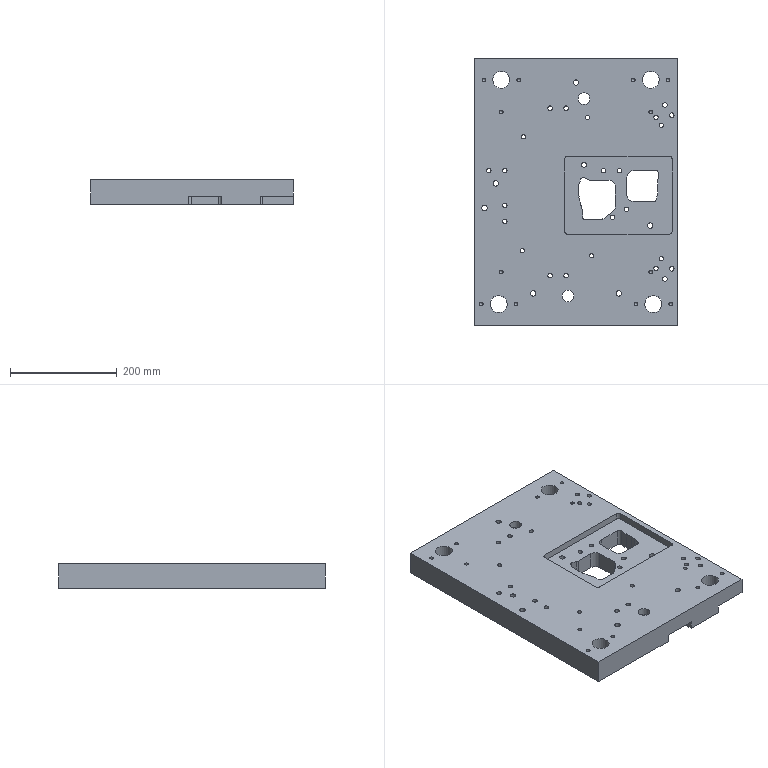Part | STEP file | 303_id634_x_t | 1 solid | 225 faces | box 380 x 500 x 45 mm | volume 7480800 mm3 | cylinder 120 | cone 51 | plane 47 | spline 7 | commonest cylinder face diameters 6.8 x32 8.5 x23 10 x17 5.2 x8 8 x8 30 x8